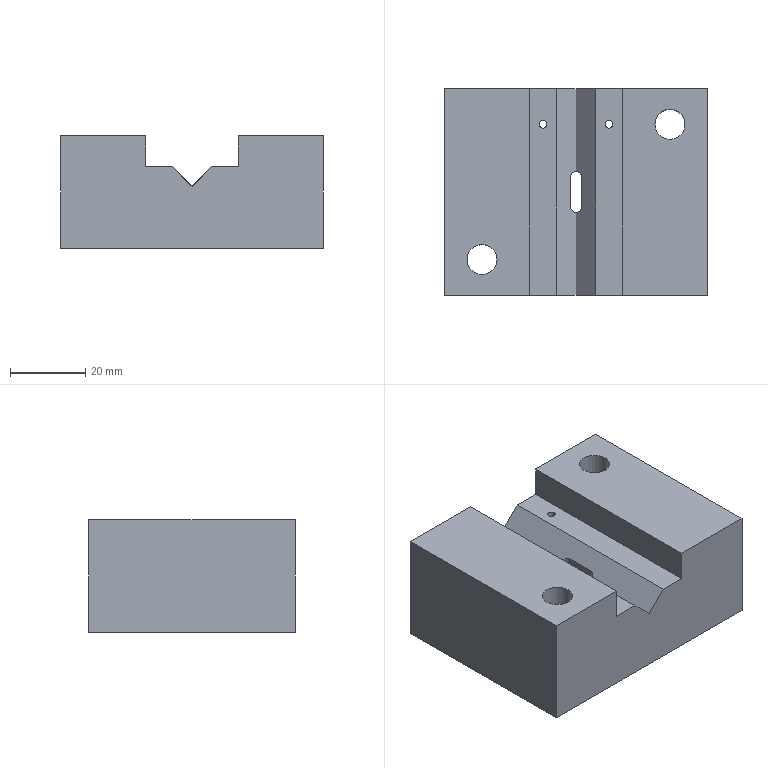Part | NX | features DATUM_CSYS 8, EXTRUDE 7, SKETCH 7, DATUM_PLANE 1 | 1 solid | 27 faces | box 70 x 55 x 30 mm | volume 96709 mm3 | plane 18 | cylinder 9 | commonest cylinder face diameters 8 x4 2 x2 3 x2 12 x1
STEP:
#1=CARTESIAN_POINT('',(-12.29,-27.5,21.757));
#2=VERTEX_POINT('',#1);
#3=CARTESIAN_POINT('',(-12.29,-27.5,30.));
#4=VERTEX_POINT('',#3);
#5=CARTESIAN_POINT('',(-12.29,-27.5,33.257));
#6=DIRECTION('',(0.,0.,-1.));
#7=VECTOR('',#6,1000.);
#8=LINE('',#5,#7);
#9=EDGE_CURVE('',#2,#4,#8,.F.);
#10=ORIENTED_EDGE('',*,*,#9,.T.);
#11=CARTESIAN_POINT('',(-35.,-27.5,30.));
#12=VERTEX_POINT('',#11);
#13=CARTESIAN_POINT('',(-35.,-27.5,30.));
#14=DIRECTION('',(1.,0.,0.));
#15=VECTOR('',#14,1000.);
#16=LINE('',#13,#15);
#17=EDGE_CURVE('',#12,#4,#16,.T.);
#18=ORIENTED_EDGE('',*,*,#17,.F.);
#19=CARTESIAN_POINT('',(-35.,-27.5,0.));
#20=VERTEX_POINT('',#19);
#21=CARTESIAN_POINT('',(-35.,-27.5,30.));
#22=DIRECTION('',(0.,0.,-1.));
#23=VECTOR('',#22,1000.);
#24=LINE('',#21,#23);
#25=EDGE_CURVE('',#12,#20,#24,.T.);
#26=ORIENTED_EDGE('',*,*,#25,.T.);
#27=CARTESIAN_POINT('',(35.,-27.5,0.));
#28=VERTEX_POINT('',#27);
#29=CARTESIAN_POINT('',(-35.,-27.5,0.));
#30=DIRECTION('',(1.,0.,0.));
#31=VECTOR('',#30,1000.);
#32=LINE('',#29,#31);
#33=EDGE_CURVE('',#20,#28,#32,.T.);
#34=ORIENTED_EDGE('',*,*,#33,.T.);
#35=CARTESIAN_POINT('',(35.,-27.5,30.));
#36=VERTEX_POINT('',#35);
#37=CARTESIAN_POINT('',(35.,-27.5,30.));
#38=DIRECTION('',(0.,0.,-1.));
#39=VECTOR('',#38,1000.);
#40=LINE('',#37,#39);
#41=EDGE_CURVE('',#36,#28,#40,.T.);
#42=ORIENTED_EDGE('',*,*,#41,.F.);
#43=CARTESIAN_POINT('',(12.29,-27.5,30.));
#44=VERTEX_POINT('',#43);
#45=CARTESIAN_POINT('',(-35.,-27.5,30.));
#46=DIRECTION('',(1.,0.,0.));
#47=VECTOR('',#46,1000.);
#48=LINE('',#45,#47);
#49=EDGE_CURVE('',#44,#36,#48,.T.);
#50=ORIENTED_EDGE('',*,*,#49,.F.);
#51=CARTESIAN_POINT('',(12.29,-27.5,21.757));
#52=VERTEX_POINT('',#51);
#53=CARTESIAN_POINT('',(12.29,-27.5,21.757));
#54=DIRECTION('',(0.,0.,1.));
#55=VECTOR('',#54,1000.);
#56=LINE('',#53,#55);
#57=EDGE_CURVE('',#44,#52,#56,.F.);
#58=ORIENTED_EDGE('',*,*,#57,.T.);
#59=CARTESIAN_POINT('',(5.29,-27.5,21.757));
#60=VERTEX_POINT('',#59);
#61=CARTESIAN_POINT('',(5.29,-27.5,21.757));
#62=DIRECTION('',(1.,0.,0.));
#63=VECTOR('',#62,1000.);
#64=LINE('',#61,#63);
#65=EDGE_CURVE('',#60,#52,#64,.T.);
#66=ORIENTED_EDGE('',*,*,#65,.F.);
#67=CARTESIAN_POINT('',(0.,-27.5,16.467));
#68=VERTEX_POINT('',#67);
#69=CARTESIAN_POINT('',(0.,-27.5,16.467));
#70=DIRECTION('',(0.7071,0.,0.7071));
#71=VECTOR('',#70,1000.);
#72=LINE('',#69,#71);
#73=EDGE_CURVE('',#68,#60,#72,.T.);
#74=ORIENTED_EDGE('',*,*,#73,.F.);
#75=CARTESIAN_POINT('',(-5.29,-27.5,21.757));
#76=VERTEX_POINT('',#75);
#77=CARTESIAN_POINT('',(-5.29,-27.5,21.757));
#78=DIRECTION('',(0.7071,0.,-0.7071));
#79=VECTOR('',#78,1000.);
#80=LINE('',#77,#79);
#81=EDGE_CURVE('',#76,#68,#80,.T.);
#82=ORIENTED_EDGE('',*,*,#81,.F.);
#83=CARTESIAN_POINT('',(-12.29,-27.5,21.757));
#84=DIRECTION('',(1.,0.,0.));
#85=VECTOR('',#84,1000.);
#86=LINE('',#83,#85);
#87=EDGE_CURVE('',#2,#76,#86,.T.);
#88=ORIENTED_EDGE('',*,*,#87,.F.);
#89=EDGE_LOOP('',(#10,#18,#26,#34,#42,#50,#58,#66,#74,#82,#88));
#90=FACE_BOUND('',#89,.T.);
#91=CARTESIAN_POINT('',(-35.,-27.5,30.));
#92=DIRECTION('',(0.,1.,0.));
#93=DIRECTION('',(-1.,0.,0.));
#94=AXIS2_PLACEMENT_3D('',#91,#92,#93);
#95=PLANE('',#94);
#96=ADVANCED_FACE('',(#90),#95,.F.);
#97=CARTESIAN_POINT('',(-21.,-18.,30.));
#98=VERTEX_POINT('',#97);
#99=CARTESIAN_POINT('',(-25.,-18.,30.));
#100=DIRECTION('',(0.,0.,1.));
#101=DIRECTION('',(1.,0.,0.));
#102=AXIS2_PLACEMENT_3D('',#99,#100,#101);
#103=CIRCLE('',#102,4.);
#104=EDGE_CURVE('',#98,#98,#103,.T.);
#105=ORIENTED_EDGE('',*,*,#104,.F.);
#106=EDGE_LOOP('',(#105));
#107=FACE_BOUND('',#106,.T.);
#108=CARTESIAN_POINT('',(-12.29,27.5,30.));
#109=VERTEX_POINT('',#108);
#110=CARTESIAN_POINT('',(-12.29,0.,30.));
#111=DIRECTION('',(0.,-1.,0.));
#112=VECTOR('',#111,1000.);
#113=LINE('',#110,#112);
#114=EDGE_CURVE('',#109,#4,#113,.T.);
#115=ORIENTED_EDGE('',*,*,#114,.F.);
#116=CARTESIAN_POINT('',(-35.,27.5,30.));
#117=VERTEX_POINT('',#116);
#118=CARTESIAN_POINT('',(35.,27.5,30.));
#119=DIRECTION('',(-1.,0.,0.));
#120=VECTOR('',#119,1000.);
#121=LINE('',#118,#120);
#122=EDGE_CURVE('',#109,#117,#121,.T.);
#123=ORIENTED_EDGE('',*,*,#122,.T.);
#124=CARTESIAN_POINT('',(-35.,27.5,30.));
#125=DIRECTION('',(0.,-1.,0.));
#126=VECTOR('',#125,1000.);
#127=LINE('',#124,#126);
#128=EDGE_CURVE('',#117,#12,#127,.T.);
#129=ORIENTED_EDGE('',*,*,#128,.T.);
#130=ORIENTED_EDGE('',*,*,#17,.T.);
#131=EDGE_LOOP('',(#115,#123,#129,#130));
#132=FACE_BOUND('',#131,.T.);
#133=CARTESIAN_POINT('',(0.,0.,30.));
#134=DIRECTION('',(0.,0.,1.));
#135=DIRECTION('',(1.,0.,0.));
#136=AXIS2_PLACEMENT_3D('',#133,#134,#135);
#137=PLANE('',#136);
#138=ADVANCED_FACE('',(#107,#132),#137,.T.);
#139=CARTESIAN_POINT('',(-1.5,-4.,17.967));
#140=VERTEX_POINT('',#139);
#141=CARTESIAN_POINT('',(-1.5,4.,17.967));
#142=VERTEX_POINT('',#141);
#143=CARTESIAN_POINT('',(-1.5,4.,17.967));
#144=DIRECTION('',(0.,1.,0.));
#145=VECTOR('',#144,1000.);
#146=LINE('',#143,#145);
#147=EDGE_CURVE('',#140,#142,#146,.T.);
#148=ORIENTED_EDGE('',*,*,#147,.F.);
#149=CARTESIAN_POINT('',(-1.5,-4.,5.));
#150=VERTEX_POINT('',#149);
#151=CARTESIAN_POINT('',(-1.5,-4.,38.4));
#152=DIRECTION('',(0.,0.,-1.));
#153=VECTOR('',#152,1000.);
#154=LINE('',#151,#153);
#155=EDGE_CURVE('',#150,#140,#154,.F.);
#156=ORIENTED_EDGE('',*,*,#155,.F.);
#157=CARTESIAN_POINT('',(-1.5,4.,5.));
#158=VERTEX_POINT('',#157);
#159=CARTESIAN_POINT('',(-1.5,4.,5.));
#160=DIRECTION('',(0.,1.,0.));
#161=VECTOR('',#160,1000.);
#162=LINE('',#159,#161);
#163=EDGE_CURVE('',#150,#158,#162,.T.);
#164=ORIENTED_EDGE('',*,*,#163,.T.);
#165=CARTESIAN_POINT('',(-1.5,4.,38.4));
#166=DIRECTION('',(0.,0.,-1.));
#167=VECTOR('',#166,1000.);
#168=LINE('',#165,#167);
#169=EDGE_CURVE('',#158,#142,#168,.F.);
#170=ORIENTED_EDGE('',*,*,#169,.T.);
#171=EDGE_LOOP('',(#148,#156,#164,#170));
#172=FACE_BOUND('',#171,.T.);
#173=CARTESIAN_POINT('',(-1.5,4.,38.4));
#174=DIRECTION('',(1.,0.,0.));
#175=DIRECTION('',(0.,1.,0.));
#176=AXIS2_PLACEMENT_3D('',#173,#174,#175);
#177=PLANE('',#176);
#178=ADVANCED_FACE('',(#172),#177,.T.);
#179=CARTESIAN_POINT('',(0.,-5.5,16.467));
#180=VERTEX_POINT('',#179);
#181=CARTESIAN_POINT('',(0.,-4.,16.467));
#182=DIRECTION('',(-0.7071,0.,-0.7071));
#183=DIRECTION('',(0.7071,0.,-0.7071));
#184=AXIS2_PLACEMENT_3D('',#181,#182,#183);
#185=ELLIPSE('',#184,2.121,1.5);
#186=EDGE_CURVE('',#180,#140,#185,.T.);
#187=ORIENTED_EDGE('',*,*,#186,.F.);
#188=CARTESIAN_POINT('',(1.5,-4.,17.967));
#189=VERTEX_POINT('',#188);
#190=CARTESIAN_POINT('',(0.,-4.,16.467));
#191=DIRECTION('',(0.7071,0.,-0.7071));
#192=DIRECTION('',(-0.7071,0.,-0.7071));
#193=AXIS2_PLACEMENT_3D('',#190,#191,#192);
#194=ELLIPSE('',#193,2.121,1.5);
#195=EDGE_CURVE('',#189,#180,#194,.T.);
#196=ORIENTED_EDGE('',*,*,#195,.F.);
#197=CARTESIAN_POINT('',(1.5,-4.,5.));
#198=VERTEX_POINT('',#197);
#199=CARTESIAN_POINT('',(1.5,-4.,38.4));
#200=DIRECTION('',(0.,0.,-1.));
#201=VECTOR('',#200,1000.);
#202=LINE('',#199,#201);
#203=EDGE_CURVE('',#198,#189,#202,.F.);
#204=ORIENTED_EDGE('',*,*,#203,.F.);
#205=CARTESIAN_POINT('',(0.,-5.5,5.));
#206=VERTEX_POINT('',#205);
#207=CARTESIAN_POINT('',(0.,-4.,5.));
#208=DIRECTION('',(0.,0.,-1.));
#209=DIRECTION('',(-1.,0.,0.));
#210=AXIS2_PLACEMENT_3D('',#207,#208,#209);
#211=CIRCLE('',#210,1.5);
#212=EDGE_CURVE('',#198,#206,#211,.T.);
#213=ORIENTED_EDGE('',*,*,#212,.T.);
#214=CARTESIAN_POINT('',(0.,-4.,5.));
#215=DIRECTION('',(0.,0.,-1.));
#216=DIRECTION('',(-1.,0.,0.));
#217=AXIS2_PLACEMENT_3D('',#214,#215,#216);
#218=CIRCLE('',#217,1.5);
#219=EDGE_CURVE('',#206,#150,#218,.T.);
#220=ORIENTED_EDGE('',*,*,#219,.T.);
#221=ORIENTED_EDGE('',*,*,#155,.T.);
#222=EDGE_LOOP('',(#187,#196,#204,#213,#220,#221));
#223=FACE_BOUND('',#222,.T.);
#224=CARTESIAN_POINT('',(0.,-4.,38.4));
#225=DIRECTION('',(0.,0.,-1.));
#226=DIRECTION('',(-1.,0.,0.));
#227=AXIS2_PLACEMENT_3D('',#224,#225,#226);
#228=CYLINDRICAL_SURFACE('',#227,1.5);
#229=ADVANCED_FACE('',(#223),#228,.F.);
#230=CARTESIAN_POINT('',(1.5,4.,17.967));
#231=VERTEX_POINT('',#230);
#232=CARTESIAN_POINT('',(1.5,-4.,17.967));
#233=DIRECTION('',(0.,-1.,0.));
#234=VECTOR('',#233,1000.);
#235=LINE('',#232,#234);
#236=EDGE_CURVE('',#231,#189,#235,.T.);
#237=ORIENTED_EDGE('',*,*,#236,.F.);
#238=CARTESIAN_POINT('',(1.5,4.,5.));
#239=VERTEX_POINT('',#238);
#240=CARTESIAN_POINT('',(1.5,4.,38.4));
#241=DIRECTION('',(0.,0.,-1.));
#242=VECTOR('',#241,1000.);
#243=LINE('',#240,#242);
#244=EDGE_CURVE('',#239,#231,#243,.F.);
#245=ORIENTED_EDGE('',*,*,#244,.F.);
#246=CARTESIAN_POINT('',(1.5,-4.,5.));
#247=DIRECTION('',(0.,-1.,0.));
#248=VECTOR('',#247,1000.);
#249=LINE('',#246,#248);
#250=EDGE_CURVE('',#239,#198,#249,.T.);
#251=ORIENTED_EDGE('',*,*,#250,.T.);
#252=ORIENTED_EDGE('',*,*,#203,.T.);
#253=EDGE_LOOP('',(#237,#245,#251,#252));
#254=FACE_BOUND('',#253,.T.);
#255=CARTESIAN_POINT('',(1.5,-4.,38.4));
#256=DIRECTION('',(-1.,0.,0.));
#257=DIRECTION('',(0.,-1.,0.));
#258=AXIS2_PLACEMENT_3D('',#255,#256,#257);
#259=PLANE('',#258);
#260=ADVANCED_FACE('',(#254),#259,.T.);
#261=CARTESIAN_POINT('',(0.,5.5,16.467));
#262=VERTEX_POINT('',#261);
#263=CARTESIAN_POINT('',(0.,4.,16.467));
#264=DIRECTION('',(-0.7071,0.,-0.7071));
#265=DIRECTION('',(0.7071,0.,-0.7071));
#266=AXIS2_PLACEMENT_3D('',#263,#264,#265);
#267=ELLIPSE('',#266,2.121,1.5);
#268=EDGE_CURVE('',#142,#262,#267,.T.);
#269=ORIENTED_EDGE('',*,*,#268,.F.);
#270=ORIENTED_EDGE('',*,*,#169,.F.);
#271=CARTESIAN_POINT('',(0.,4.,5.));
#272=DIRECTION('',(0.,0.,-1.));
#273=DIRECTION('',(-1.,0.,0.));
#274=AXIS2_PLACEMENT_3D('',#271,#272,#273);
#275=CIRCLE('',#274,1.5);
#276=EDGE_CURVE('',#158,#239,#275,.T.);
#277=ORIENTED_EDGE('',*,*,#276,.T.);
#278=ORIENTED_EDGE('',*,*,#244,.T.);
#279=CARTESIAN_POINT('',(0.,4.,16.467));
#280=DIRECTION('',(0.7071,0.,-0.7071));
#281=DIRECTION('',(-0.7071,0.,-0.7071));
#282=AXIS2_PLACEMENT_3D('',#279,#280,#281);
#283=ELLIPSE('',#282,2.121,1.5);
#284=EDGE_CURVE('',#262,#231,#283,.T.);
#285=ORIENTED_EDGE('',*,*,#284,.F.);
#286=EDGE_LOOP('',(#269,#270,#277,#278,#285));
#287=FACE_BOUND('',#286,.T.);
#288=CARTESIAN_POINT('',(0.,4.,38.4));
#289=DIRECTION('',(0.,0.,-1.));
#290=DIRECTION('',(-1.,0.,0.));
#291=AXIS2_PLACEMENT_3D('',#288,#289,#290);
#292=CYLINDRICAL_SURFACE('',#291,1.5);
#293=ADVANCED_FACE('',(#287),#292,.F.);
#294=CARTESIAN_POINT('',(-35.,27.5,0.));
#295=VERTEX_POINT('',#294);
#296=CARTESIAN_POINT('',(-35.,27.5,0.));
#297=DIRECTION('',(0.,-1.,0.));
#298=VECTOR('',#297,1000.);
#299=LINE('',#296,#298);
#300=EDGE_CURVE('',#295,#20,#299,.T.);
#301=ORIENTED_EDGE('',*,*,#300,.T.);
#302=ORIENTED_EDGE('',*,*,#25,.F.);
#303=ORIENTED_EDGE('',*,*,#128,.F.);
#304=CARTESIAN_POINT('',(-35.,27.5,30.));
#305=DIRECTION('',(0.,0.,-1.));
#306=VECTOR('',#305,1000.);
#307=LINE('',#304,#306);
#308=EDGE_CURVE('',#117,#295,#307,.T.);
#309=ORIENTED_EDGE('',*,*,#308,.T.);
#310=EDGE_LOOP('',(#301,#302,#303,#309));
#311=FACE_BOUND('',#310,.T.);
#312=CARTESIAN_POINT('',(-35.,27.5,30.));
#313=DIRECTION('',(1.,0.,0.));
#314=DIRECTION('',(0.,0.,-1.));
#315=AXIS2_PLACEMENT_3D('',#312,#313,#314);
#316=PLANE('',#315);
#317=ADVANCED_FACE('',(#311),#316,.F.);
#318=CARTESIAN_POINT('',(35.,27.5,0.));
#319=VERTEX_POINT('',#318);
#320=CARTESIAN_POINT('',(35.,-27.5,0.));
#321=DIRECTION('',(0.,1.,0.));
#322=VECTOR('',#321,1000.);
#323=LINE('',#320,#322);
#324=EDGE_CURVE('',#28,#319,#323,.T.);
#325=ORIENTED_EDGE('',*,*,#324,.T.);
#326=CARTESIAN_POINT('',(35.,27.5,30.));
#327=VERTEX_POINT('',#326);
#328=CARTESIAN_POINT('',(35.,27.5,30.));
#329=DIRECTION('',(0.,0.,-1.));
#330=VECTOR('',#329,1000.);
#331=LINE('',#328,#330);
#332=EDGE_CURVE('',#327,#319,#331,.T.);
#333=ORIENTED_EDGE('',*,*,#332,.F.);
#334=CARTESIAN_POINT('',(35.,-27.5,30.));
#335=DIRECTION('',(0.,1.,0.));
#336=VECTOR('',#335,1000.);
#337=LINE('',#334,#336);
#338=EDGE_CURVE('',#36,#327,#337,.T.);
#339=ORIENTED_EDGE('',*,*,#338,.F.);
#340=ORIENTED_EDGE('',*,*,#41,.T.);
#341=EDGE_LOOP('',(#325,#333,#339,#340));
#342=FACE_BOUND('',#341,.T.);
#343=CARTESIAN_POINT('',(35.,-27.5,30.));
#344=DIRECTION('',(-1.,0.,0.));
#345=DIRECTION('',(0.,-1.,0.));
#346=AXIS2_PLACEMENT_3D('',#343,#344,#345);
#347=PLANE('',#346);
#348=ADVANCED_FACE('',(#342),#347,.F.);
#349=ORIENTED_EDGE('',*,*,#122,.F.);
#350=CARTESIAN_POINT('',(-12.29,27.5,21.757));
#351=VERTEX_POINT('',#350);
#352=CARTESIAN_POINT('',(-12.29,27.5,30.));
#353=DIRECTION('',(0.,0.,-1.));
#354=VECTOR('',#353,1000.);
#355=LINE('',#352,#354);
#356=EDGE_CURVE('',#109,#351,#355,.T.);
#357=ORIENTED_EDGE('',*,*,#356,.T.);
#358=CARTESIAN_POINT('',(-5.29,27.5,21.757));
#359=VERTEX_POINT('',#358);
#360=CARTESIAN_POINT('',(35.,27.5,21.757));
#361=DIRECTION('',(1.,0.,0.));
#362=VECTOR('',#361,1000.);
#363=LINE('',#360,#362);
#364=EDGE_CURVE('',#351,#359,#363,.T.);
#365=ORIENTED_EDGE('',*,*,#364,.T.);
#366=CARTESIAN_POINT('',(0.,27.5,16.467));
#367=VERTEX_POINT('',#366);
#368=CARTESIAN_POINT('',(10.733,27.5,5.733));
#369=DIRECTION('',(0.7071,0.,-0.7071));
#370=VECTOR('',#369,1000.);
#371=LINE('',#368,#370);
#372=EDGE_CURVE('',#359,#367,#371,.T.);
#373=ORIENTED_EDGE('',*,*,#372,.T.);
#374=CARTESIAN_POINT('',(5.29,27.5,21.757));
#375=VERTEX_POINT('',#374);
#376=CARTESIAN_POINT('',(24.267,27.5,40.733));
#377=DIRECTION('',(0.7071,0.,0.7071));
#378=VECTOR('',#377,1000.);
#379=LINE('',#376,#378);
#380=EDGE_CURVE('',#367,#375,#379,.T.);
#381=ORIENTED_EDGE('',*,*,#380,.T.);
#382=CARTESIAN_POINT('',(12.29,27.5,21.757));
#383=VERTEX_POINT('',#382);
#384=CARTESIAN_POINT('',(35.,27.5,21.757));
#385=DIRECTION('',(1.,0.,0.));
#386=VECTOR('',#385,1000.);
#387=LINE('',#384,#386);
#388=EDGE_CURVE('',#375,#383,#387,.T.);
#389=ORIENTED_EDGE('',*,*,#388,.T.);
#390=CARTESIAN_POINT('',(12.29,27.5,30.));
#391=VERTEX_POINT('',#390);
#392=CARTESIAN_POINT('',(12.29,27.5,30.));
#393=DIRECTION('',(0.,0.,1.));
#394=VECTOR('',#393,1000.);
#395=LINE('',#392,#394);
#396=EDGE_CURVE('',#383,#391,#395,.T.);
#397=ORIENTED_EDGE('',*,*,#396,.T.);
#398=CARTESIAN_POINT('',(35.,27.5,30.));
#399=DIRECTION('',(-1.,0.,0.));
#400=VECTOR('',#399,1000.);
#401=LINE('',#398,#400);
#402=EDGE_CURVE('',#327,#391,#401,.T.);
#403=ORIENTED_EDGE('',*,*,#402,.F.);
#404=ORIENTED_EDGE('',*,*,#332,.T.);
#405=CARTESIAN_POINT('',(35.,27.5,0.));
#406=DIRECTION('',(-1.,0.,0.));
#407=VECTOR('',#406,1000.);
#408=LINE('',#405,#407);
#409=EDGE_CURVE('',#319,#295,#408,.T.);
#410=ORIENTED_EDGE('',*,*,#409,.T.);
#411=ORIENTED_EDGE('',*,*,#308,.F.);
#412=EDGE_LOOP('',(#349,#357,#365,#373,#381,#389,#397,#403,#404,#410,#411));
#413=FACE_BOUND('',#412,.T.);
#414=CARTESIAN_POINT('',(35.,27.5,30.));
#415=DIRECTION('',(0.,-1.,0.));
#416=DIRECTION('',(1.,0.,0.));
#417=AXIS2_PLACEMENT_3D('',#414,#415,#416);
#418=PLANE('',#417);
#419=ADVANCED_FACE('',(#413),#418,.F.);
#420=CARTESIAN_POINT('',(29.,18.,30.));
#421=VERTEX_POINT('',#420);
#422=CARTESIAN_POINT('',(25.,18.,30.));
#423=DIRECTION('',(0.,0.,1.));
#424=DIRECTION('',(1.,0.,0.));
#425=AXIS2_PLACEMENT_3D('',#422,#423,#424);
#426=CIRCLE('',#425,4.);
#427=EDGE_CURVE('',#421,#421,#426,.T.);
#428=ORIENTED_EDGE('',*,*,#427,.F.);
#429=EDGE_LOOP('',(#428));
#430=FACE_BOUND('',#429,.T.);
#431=CARTESIAN_POINT('',(12.29,0.,30.));
#432=DIRECTION('',(0.,1.,0.));
#433=VECTOR('',#432,1000.);
#434=LINE('',#431,#433);
#435=EDGE_CURVE('',#44,#391,#434,.T.);
#436=ORIENTED_EDGE('',*,*,#435,.F.);
#437=ORIENTED_EDGE('',*,*,#49,.T.);
#438=ORIENTED_EDGE('',*,*,#338,.T.);
#439=ORIENTED_EDGE('',*,*,#402,.T.);
#440=EDGE_LOOP('',(#436,#437,#438,#439));
#441=FACE_BOUND('',#440,.T.);
#442=CARTESIAN_POINT('',(0.,0.,30.));
#443=DIRECTION('',(0.,0.,1.));
#444=DIRECTION('',(1.,0.,0.));
#445=AXIS2_PLACEMENT_3D('',#442,#443,#444);
#446=PLANE('',#445);
#447=ADVANCED_FACE('',(#430,#441),#446,.T.);
#448=CARTESIAN_POINT('',(-7.79,18.,0.));
#449=VERTEX_POINT('',#448);
#450=CARTESIAN_POINT('',(-8.79,18.,0.));
#451=DIRECTION('',(0.,0.,1.));
#452=DIRECTION('',(1.,0.,0.));
#453=AXIS2_PLACEMENT_3D('',#450,#451,#452);
#454=CIRCLE('',#453,1.);
#455=EDGE_CURVE('',#449,#449,#454,.F.);
#456=ORIENTED_EDGE('',*,*,#455,.F.);
#457=EDGE_LOOP('',(#456));
#458=FACE_BOUND('',#457,.T.);
#459=CARTESIAN_POINT('',(9.79,18.,0.));
#460=VERTEX_POINT('',#459);
#461=CARTESIAN_POINT('',(8.79,18.,0.));
#462=DIRECTION('',(0.,0.,1.));
#463=DIRECTION('',(1.,0.,0.));
#464=AXIS2_PLACEMENT_3D('',#461,#462,#463);
#465=CIRCLE('',#464,1.);
#466=EDGE_CURVE('',#460,#460,#465,.T.);
#467=ORIENTED_EDGE('',*,*,#466,.T.);
#468=EDGE_LOOP('',(#467));
#469=FACE_BOUND('',#468,.T.);
#470=CARTESIAN_POINT('',(29.5,-18.,0.));
#471=VERTEX_POINT('',#470);
#472=CARTESIAN_POINT('',(25.5,-18.,0.));
#473=DIRECTION('',(0.,0.,-1.));
#474=DIRECTION('',(1.,0.,0.));
#475=AXIS2_PLACEMENT_3D('',#472,#473,#474);
#476=CIRCLE('',#475,4.);
#477=EDGE_CURVE('',#471,#471,#476,.T.);
#478=ORIENTED_EDGE('',*,*,#477,.F.);
#479=EDGE_LOOP('',(#478));
#480=FACE_BOUND('',#479,.T.);
#481=CARTESIAN_POINT('',(-21.,18.,0.));
#482=VERTEX_POINT('',#481);
#483=CARTESIAN_POINT('',(-25.,18.,0.));
#484=DIRECTION('',(0.,0.,-1.));
#485=DIRECTION('',(1.,0.,0.));
#486=AXIS2_PLACEMENT_3D('',#483,#484,#485);
#487=CIRCLE('',#486,4.);
#488=EDGE_CURVE('',#482,#482,#487,.T.);
#489=ORIENTED_EDGE('',*,*,#488,.F.);
#490=EDGE_LOOP('',(#489));
#491=FACE_BOUND('',#490,.T.);
#492=CARTESIAN_POINT('',(21.,18.,0.));
#493=VERTEX_POINT('',#492);
#494=CARTESIAN_POINT('',(25.,18.,0.));
#495=DIRECTION('',(0.,0.,-1.));
#496=DIRECTION('',(-1.,0.,0.));
#497=AXIS2_PLACEMENT_3D('',#494,#495,#496);
#498=CIRCLE('',#497,4.);
#499=EDGE_CURVE('',#493,#493,#498,.T.);
#500=ORIENTED_EDGE('',*,*,#499,.F.);
#501=EDGE_LOOP('',(#500));
#502=FACE_BOUND('',#501,.T.);
#503=CARTESIAN_POINT('',(-29.,-18.,0.));
#504=VERTEX_POINT('',#503);
#505=CARTESIAN_POINT('',(-25.,-18.,0.));
#506=DIRECTION('',(0.,0.,-1.));
#507=DIRECTION('',(-1.,0.,0.));
#508=AXIS2_PLACEMENT_3D('',#505,#506,#507);
#509=CIRCLE('',#508,4.);
#510=EDGE_CURVE('',#504,#504,#509,.T.);
#511=ORIENTED_EDGE('',*,*,#510,.F.);
#512=EDGE_LOOP('',(#511));
#513=FACE_BOUND('',#512,.T.);
#514=CARTESIAN_POINT('',(6.,0.5,0.));
#515=VERTEX_POINT('',#514);
#516=CARTESIAN_POINT('',(0.,0.5,0.));
#517=DIRECTION('',(0.,0.,1.));
#518=DIRECTION('',(1.,0.,0.));
#519=AXIS2_PLACEMENT_3D('',#516,#517,#518);
#520=CIRCLE('',#519,6.);
#521=EDGE_CURVE('',#515,#515,#520,.F.);
#522=ORIENTED_EDGE('',*,*,#521,.F.);
#523=EDGE_LOOP('',(#522));
#524=FACE_BOUND('',#523,.T.);
#525=ORIENTED_EDGE('',*,*,#300,.F.);
#526=ORIENTED_EDGE('',*,*,#409,.F.);
#527=ORIENTED_EDGE('',*,*,#324,.F.);
#528=ORIENTED_EDGE('',*,*,#33,.F.);
#529=EDGE_LOOP('',(#525,#526,#527,#528));
#530=FACE_BOUND('',#529,.T.);
#531=CARTESIAN_POINT('',(0.,0.,0.));
#532=DIRECTION('',(0.,0.,1.));
#533=DIRECTION('',(1.,0.,0.));
#534=AXIS2_PLACEMENT_3D('',#531,#532,#533);
#535=PLANE('',#534);
#536=ADVANCED_FACE('',(#458,#469,#480,#491,#502,#513,#524,#530),#535,.F.);
#537=CARTESIAN_POINT('',(0.,0.5,5.));
#538=DIRECTION('',(0.,0.,-1.));
#539=DIRECTION('',(1.,0.,0.));
#540=AXIS2_PLACEMENT_3D('',#537,#538,#539);
#541=CIRCLE('',#540,6.);
#542=EDGE_CURVE('',#206,#206,#541,.F.);
#543=ORIENTED_EDGE('',*,*,#542,.T.);
#544=EDGE_LOOP('',(#543));
#545=FACE_BOUND('',#544,.T.);
#546=ORIENTED_EDGE('',*,*,#521,.T.);
#547=EDGE_LOOP('',(#546));
#548=FACE_BOUND('',#547,.T.);
#549=CARTESIAN_POINT('',(0.,0.5,-25.));
#550=DIRECTION('',(0.,0.,1.));
#551=DIRECTION('',(1.,0.,0.));
#552=AXIS2_PLACEMENT_3D('',#549,#550,#551);
#553=CYLINDRICAL_SURFACE('',#552,6.);
#554=ADVANCED_FACE('',(#545,#548),#553,.F.);
#555=ORIENTED_EDGE('',*,*,#219,.F.);
#556=ORIENTED_EDGE('',*,*,#542,.F.);
#557=ORIENTED_EDGE('',*,*,#212,.F.);
#558=ORIENTED_EDGE('',*,*,#250,.F.);
#559=ORIENTED_EDGE('',*,*,#276,.F.);
#560=ORIENTED_EDGE('',*,*,#163,.F.);
#561=EDGE_LOOP('',(#555,#556,#557,#558,#559,#560));
#562=FACE_BOUND('',#561,.T.);
#563=CARTESIAN_POINT('',(0.,0.5,5.));
#564=DIRECTION('',(0.,0.,-1.));
#565=DIRECTION('',(-1.,0.,0.));
#566=AXIS2_PLACEMENT_3D('',#563,#564,#565);
#567=PLANE('',#566);
#568=ADVANCED_FACE('',(#562),#567,.T.);
#569=CARTESIAN_POINT('',(-9.79,18.,21.757));
#570=VERTEX_POINT('',#569);
#571=CARTESIAN_POINT('',(-8.79,18.,21.757));
#572=DIRECTION('',(0.,0.,-1.));
#573=DIRECTION('',(-1.,0.,0.));
#574=AXIS2_PLACEMENT_3D('',#571,#572,#573);
#575=CIRCLE('',#574,1.);
#576=EDGE_CURVE('',#570,#570,#575,.T.);
#577=ORIENTED_EDGE('',*,*,#576,.T.);
#578=EDGE_LOOP('',(#577));
#579=FACE_BOUND('',#578,.T.);
#580=CARTESIAN_POINT('',(-12.29,29.5,21.757));
#581=DIRECTION('',(0.,-1.,0.));
#582=VECTOR('',#581,1000.);
#583=LINE('',#580,#582);
#584=EDGE_CURVE('',#2,#351,#583,.F.);
#585=ORIENTED_EDGE('',*,*,#584,.F.);
#586=ORIENTED_EDGE('',*,*,#87,.T.);
#587=CARTESIAN_POINT('',(-5.29,29.5,21.757));
#588=DIRECTION('',(0.,-1.,0.));
#589=VECTOR('',#588,1000.);
#590=LINE('',#587,#589);
#591=EDGE_CURVE('',#76,#359,#590,.F.);
#592=ORIENTED_EDGE('',*,*,#591,.T.);
#593=ORIENTED_EDGE('',*,*,#364,.F.);
#594=EDGE_LOOP('',(#585,#586,#592,#593));
#595=FACE_BOUND('',#594,.T.);
#596=CARTESIAN_POINT('',(-12.29,29.5,21.757));
#597=DIRECTION('',(0.,0.,-1.));
#598=DIRECTION('',(-1.,0.,0.));
#599=AXIS2_PLACEMENT_3D('',#596,#597,#598);
#600=PLANE('',#599);
#601=ADVANCED_FACE('',(#579,#595),#600,.F.);
#602=ORIENTED_EDGE('',*,*,#186,.T.);
#603=ORIENTED_EDGE('',*,*,#147,.T.);
#604=ORIENTED_EDGE('',*,*,#268,.T.);
#605=CARTESIAN_POINT('',(0.,29.5,16.467));
#606=DIRECTION('',(0.,-1.,0.));
#607=VECTOR('',#606,1000.);
#608=LINE('',#605,#607);
#609=EDGE_CURVE('',#262,#367,#608,.F.);
#610=ORIENTED_EDGE('',*,*,#609,.T.);
#611=ORIENTED_EDGE('',*,*,#372,.F.);
#612=ORIENTED_EDGE('',*,*,#591,.F.);
#613=ORIENTED_EDGE('',*,*,#81,.T.);
#614=CARTESIAN_POINT('',(0.,29.5,16.467));
#615=DIRECTION('',(0.,-1.,0.));
#616=VECTOR('',#615,1000.);
#617=LINE('',#614,#616);
#618=EDGE_CURVE('',#68,#180,#617,.F.);
#619=ORIENTED_EDGE('',*,*,#618,.T.);
#620=EDGE_LOOP('',(#602,#603,#604,#610,#611,#612,#613,#619));
#621=FACE_BOUND('',#620,.T.);
#622=CARTESIAN_POINT('',(-5.29,29.5,21.757));
#623=DIRECTION('',(-0.7071,0.,-0.7071));
#624=DIRECTION('',(-0.7071,0.,0.7071));
#625=AXIS2_PLACEMENT_3D('',#622,#623,#624);
#626=PLANE('',#625);
#627=ADVANCED_FACE('',(#621),#626,.F.);
#628=ORIENTED_EDGE('',*,*,#195,.T.);
#629=ORIENTED_EDGE('',*,*,#618,.F.);
#630=ORIENTED_EDGE('',*,*,#73,.T.);
#631=CARTESIAN_POINT('',(5.29,29.5,21.757));
#632=DIRECTION('',(0.,-1.,0.));
#633=VECTOR('',#632,1000.);
#634=LINE('',#631,#633);
#635=EDGE_CURVE('',#60,#375,#634,.F.);
#636=ORIENTED_EDGE('',*,*,#635,.T.);
#637=ORIENTED_EDGE('',*,*,#380,.F.);
#638=ORIENTED_EDGE('',*,*,#609,.F.);
#639=ORIENTED_EDGE('',*,*,#284,.T.);
#640=ORIENTED_EDGE('',*,*,#236,.T.);
#641=EDGE_LOOP('',(#628,#629,#630,#636,#637,#638,#639,#640));
#642=FACE_BOUND('',#641,.T.);
#643=CARTESIAN_POINT('',(0.,29.5,16.467));
#644=DIRECTION('',(0.7071,0.,-0.7071));
#645=DIRECTION('',(-0.7071,0.,-0.7071));
#646=AXIS2_PLACEMENT_3D('',#643,#644,#645);
#647=PLANE('',#646);
#648=ADVANCED_FACE('',(#642),#647,.F.);
#649=CARTESIAN_POINT('',(9.79,18.,21.757));
#650=VERTEX_POINT('',#649);
#651=CARTESIAN_POINT('',(8.79,18.,21.757));
#652=DIRECTION('',(0.,0.,1.));
#653=DIRECTION('',(1.,0.,0.));
#654=AXIS2_PLACEMENT_3D('',#651,#652,#653);
#655=CIRCLE('',#654,1.);
#656=EDGE_CURVE('',#650,#650,#655,.T.);
#657=ORIENTED_EDGE('',*,*,#656,.F.);
#658=EDGE_LOOP('',(#657));
#659=FACE_BOUND('',#658,.T.);
#660=ORIENTED_EDGE('',*,*,#635,.F.);
#661=ORIENTED_EDGE('',*,*,#65,.T.);
#662=CARTESIAN_POINT('',(12.29,29.5,21.757));
#663=DIRECTION('',(0.,-1.,0.));
#664=VECTOR('',#663,1000.);
#665=LINE('',#662,#664);
#666=EDGE_CURVE('',#52,#383,#665,.F.);
#667=ORIENTED_EDGE('',*,*,#666,.T.);
#668=ORIENTED_EDGE('',*,*,#388,.F.);
#669=EDGE_LOOP('',(#660,#661,#667,#668));
#670=FACE_BOUND('',#669,.T.);
#671=CARTESIAN_POINT('',(5.29,29.5,21.757));
#672=DIRECTION('',(0.,0.,-1.));
#673=DIRECTION('',(-1.,0.,0.));
#674=AXIS2_PLACEMENT_3D('',#671,#672,#673);
#675=PLANE('',#674);
#676=ADVANCED_FACE('',(#659,#670),#675,.F.);
#677=ORIENTED_EDGE('',*,*,#114,.T.);
#678=ORIENTED_EDGE('',*,*,#9,.F.);
#679=ORIENTED_EDGE('',*,*,#584,.T.);
#680=ORIENTED_EDGE('',*,*,#356,.F.);
#681=EDGE_LOOP('',(#677,#678,#679,#680));
#682=FACE_BOUND('',#681,.T.);
#683=CARTESIAN_POINT('',(-12.29,29.5,33.257));
#684=DIRECTION('',(-1.,0.,0.));
#685=DIRECTION('',(0.,0.,1.));
#686=AXIS2_PLACEMENT_3D('',#683,#684,#685);
#687=PLANE('',#686);
#688=ADVANCED_FACE('',(#682),#687,.F.);
#689=ORIENTED_EDGE('',*,*,#666,.F.);
#690=ORIENTED_EDGE('',*,*,#57,.F.);
#691=ORIENTED_EDGE('',*,*,#435,.T.);
#692=ORIENTED_EDGE('',*,*,#396,.F.);
#693=EDGE_LOOP('',(#689,#690,#691,#692));
#694=FACE_BOUND('',#693,.T.);
#695=CARTESIAN_POINT('',(12.29,29.5,21.757));
#696=DIRECTION('',(1.,0.,0.));
#697=DIRECTION('',(0.,0.,-1.));
#698=AXIS2_PLACEMENT_3D('',#695,#696,#697);
#699=PLANE('',#698);
#700=ADVANCED_FACE('',(#694),#699,.F.);
#701=ORIENTED_EDGE('',*,*,#104,.T.);
#702=EDGE_LOOP('',(#701));
#703=FACE_BOUND('',#702,.T.);
#704=ORIENTED_EDGE('',*,*,#510,.T.);
#705=EDGE_LOOP('',(#704));
#706=FACE_BOUND('',#705,.T.);
#707=CARTESIAN_POINT('',(-25.,-18.,100.));
#708=DIRECTION('',(0.,0.,-1.));
#709=DIRECTION('',(-1.,0.,0.));
#710=AXIS2_PLACEMENT_3D('',#707,#708,#709);
#711=CYLINDRICAL_SURFACE('',#710,4.);
#712=ADVANCED_FACE('',(#703,#706),#711,.F.);
#713=ORIENTED_EDGE('',*,*,#427,.T.);
#714=EDGE_LOOP('',(#713));
#715=FACE_BOUND('',#714,.T.);
#716=ORIENTED_EDGE('',*,*,#499,.T.);
#717=EDGE_LOOP('',(#716));
#718=FACE_BOUND('',#717,.T.);
#719=CARTESIAN_POINT('',(25.,18.,100.));
#720=DIRECTION('',(0.,0.,-1.));
#721=DIRECTION('',(-1.,0.,0.));
#722=AXIS2_PLACEMENT_3D('',#719,#720,#721);
#723=CYLINDRICAL_SURFACE('',#722,4.);
#724=ADVANCED_FACE('',(#715,#718),#723,.F.);
#725=CARTESIAN_POINT('',(-21.,18.,20.));
#726=VERTEX_POINT('',#725);
#727=CARTESIAN_POINT('',(-25.,18.,20.));
#728=DIRECTION('',(0.,0.,-1.));
#729=DIRECTION('',(1.,0.,0.));
#730=AXIS2_PLACEMENT_3D('',#727,#728,#729);
#731=CIRCLE('',#730,4.);
#732=EDGE_CURVE('',#726,#726,#731,.F.);
#733=ORIENTED_EDGE('',*,*,#732,.T.);
#734=EDGE_LOOP('',(#733));
#735=FACE_BOUND('',#734,.T.);
#736=ORIENTED_EDGE('',*,*,#488,.T.);
#737=EDGE_LOOP('',(#736));
#738=FACE_BOUND('',#737,.T.);
#739=CARTESIAN_POINT('',(-25.,18.,20.));
#740=DIRECTION('',(0.,0.,-1.));
#741=DIRECTION('',(-1.,0.,0.));
#742=AXIS2_PLACEMENT_3D('',#739,#740,#741);
#743=CYLINDRICAL_SURFACE('',#742,4.);
#744=ADVANCED_FACE('',(#735,#738),#743,.F.);
#745=ORIENTED_EDGE('',*,*,#732,.F.);
#746=EDGE_LOOP('',(#745));
#747=FACE_BOUND('',#746,.T.);
#748=CARTESIAN_POINT('',(-25.,18.,20.));
#749=DIRECTION('',(0.,0.,-1.));
#750=DIRECTION('',(-1.,0.,0.));
#751=AXIS2_PLACEMENT_3D('',#748,#749,#750);
#752=PLANE('',#751);
#753=ADVANCED_FACE('',(#747),#752,.T.);
#754=CARTESIAN_POINT('',(29.5,-18.,20.));
#755=VERTEX_POINT('',#754);
#756=CARTESIAN_POINT('',(25.5,-18.,20.));
#757=DIRECTION('',(0.,0.,-1.));
#758=DIRECTION('',(1.,0.,0.));
#759=AXIS2_PLACEMENT_3D('',#756,#757,#758);
#760=CIRCLE('',#759,4.);
#761=EDGE_CURVE('',#755,#755,#760,.F.);
#762=ORIENTED_EDGE('',*,*,#761,.T.);
#763=EDGE_LOOP('',(#762));
#764=FACE_BOUND('',#763,.T.);
#765=ORIENTED_EDGE('',*,*,#477,.T.);
#766=EDGE_LOOP('',(#765));
#767=FACE_BOUND('',#766,.T.);
#768=CARTESIAN_POINT('',(25.5,-18.,20.));
#769=DIRECTION('',(0.,0.,-1.));
#770=DIRECTION('',(-1.,0.,0.));
#771=AXIS2_PLACEMENT_3D('',#768,#769,#770);
#772=CYLINDRICAL_SURFACE('',#771,4.);
#773=ADVANCED_FACE('',(#764,#767),#772,.F.);
#774=ORIENTED_EDGE('',*,*,#761,.F.);
#775=EDGE_LOOP('',(#774));
#776=FACE_BOUND('',#775,.T.);
#777=CARTESIAN_POINT('',(25.5,-18.,20.));
#778=DIRECTION('',(0.,0.,-1.));
#779=DIRECTION('',(-1.,0.,0.));
#780=AXIS2_PLACEMENT_3D('',#777,#778,#779);
#781=PLANE('',#780);
#782=ADVANCED_FACE('',(#776),#781,.T.);
#783=ORIENTED_EDGE('',*,*,#656,.T.);
#784=EDGE_LOOP('',(#783));
#785=FACE_BOUND('',#784,.T.);
#786=ORIENTED_EDGE('',*,*,#466,.F.);
#787=EDGE_LOOP('',(#786));
#788=FACE_BOUND('',#787,.T.);
#789=CARTESIAN_POINT('',(8.79,18.,-7.243));
#790=DIRECTION('',(0.,0.,1.));
#791=DIRECTION('',(1.,0.,0.));
#792=AXIS2_PLACEMENT_3D('',#789,#790,#791);
#793=CYLINDRICAL_SURFACE('',#792,1.);
#794=ADVANCED_FACE('',(#785,#788),#793,.F.);
#795=ORIENTED_EDGE('',*,*,#576,.F.);
#796=EDGE_LOOP('',(#795));
#797=FACE_BOUND('',#796,.T.);
#798=ORIENTED_EDGE('',*,*,#455,.T.);
#799=EDGE_LOOP('',(#798));
#800=FACE_BOUND('',#799,.T.);
#801=CARTESIAN_POINT('',(-8.79,18.,-7.243));
#802=DIRECTION('',(0.,0.,1.));
#803=DIRECTION('',(1.,0.,0.));
#804=AXIS2_PLACEMENT_3D('',#801,#802,#803);
#805=CYLINDRICAL_SURFACE('',#804,1.);
#806=ADVANCED_FACE('',(#797,#800),#805,.F.);
#807=CLOSED_SHELL('',(#96,#138,#178,#229,#260,#293,#317,#348,#419,#447,#536,#554,#568,#601,#627,#648,#676,#688,#700,#712,#724,#744,#753,#773,#782,#794,#806));
#808=MANIFOLD_SOLID_BREP('',#807);
#809=(LENGTH_UNIT()NAMED_UNIT(*)SI_UNIT(.MILLI.,.METRE.));
#810=UNCERTAINTY_MEASURE_WITH_UNIT(LENGTH_MEASURE(0.00001),#809,'','');
#811=(NAMED_UNIT(*)PLANE_ANGLE_UNIT()SI_UNIT($,.RADIAN.));
#812=(NAMED_UNIT(*)SI_UNIT($,.STERADIAN.)SOLID_ANGLE_UNIT());
#813=(GEOMETRIC_REPRESENTATION_CONTEXT(3)GLOBAL_UNCERTAINTY_ASSIGNED_CONTEXT((#810))GLOBAL_UNIT_ASSIGNED_CONTEXT((#809,#811,#812))REPRESENTATION_CONTEXT('',''));
#814=ADVANCED_BREP_SHAPE_REPRESENTATION('',(#808),#813);